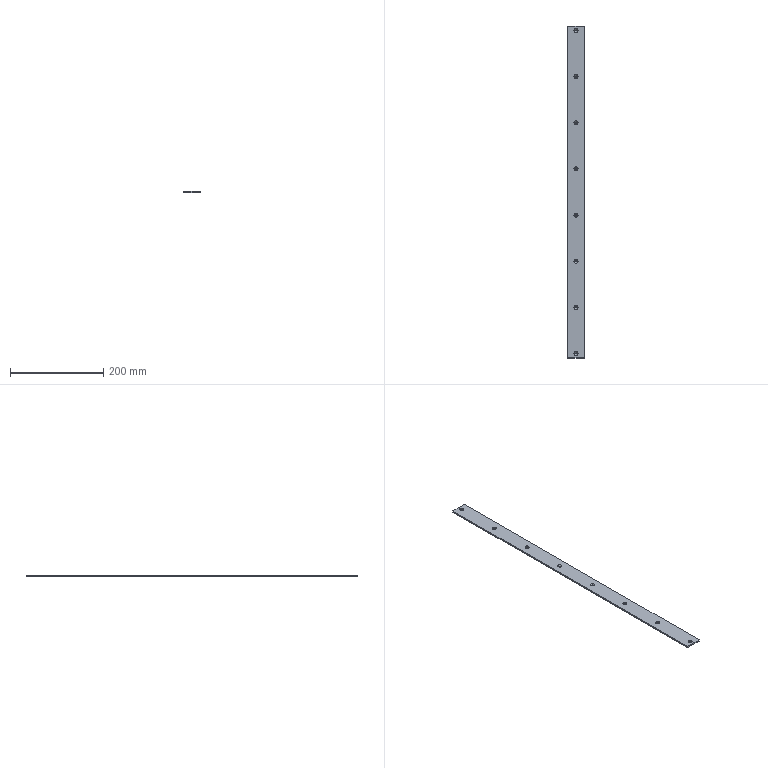Part | SolidWorks | features BaseBody 1 | 1 solid | 38 faces | box 35 x 712 x 3.2 mm | volume 79027 mm3 | cylinder 16 | cone 16 | plane 6 | commonest cylinder face diameters 4.5 x16
STEP:
#1=CARTESIAN_POINT('',(15.25,702.5,-3.2));
#2=VERTEX_POINT('',#1);
#3=CARTESIAN_POINT('',(19.75,702.5,-3.2));
#4=VERTEX_POINT('',#3);
#5=CARTESIAN_POINT('',(17.5,702.5,-3.2));
#6=DIRECTION('',(0.,0.,1.));
#7=DIRECTION('',(1.,0.,0.));
#8=AXIS2_PLACEMENT_3D('',#5,#6,#7);
#9=CIRCLE('',#8,2.25);
#10=EDGE_CURVE('',#2,#4,#9,.T.);
#11=ORIENTED_EDGE('',*,*,#10,.F.);
#12=CARTESIAN_POINT('',(15.25,702.5,-2.05));
#13=VERTEX_POINT('',#12);
#14=CARTESIAN_POINT('',(15.25,702.5,0.));
#15=DIRECTION('',(0.,0.,1.));
#16=VECTOR('',#15,1000.);
#17=LINE('',#14,#16);
#18=EDGE_CURVE('',#2,#13,#17,.T.);
#19=ORIENTED_EDGE('',*,*,#18,.T.);
#20=CARTESIAN_POINT('',(19.75,702.5,-2.05));
#21=VERTEX_POINT('',#20);
#22=CARTESIAN_POINT('',(17.5,702.5,-2.05));
#23=DIRECTION('',(0.,0.,-1.));
#24=DIRECTION('',(1.,0.,0.));
#25=AXIS2_PLACEMENT_3D('',#22,#23,#24);
#26=CIRCLE('',#25,2.25);
#27=EDGE_CURVE('',#21,#13,#26,.T.);
#28=ORIENTED_EDGE('',*,*,#27,.F.);
#29=CARTESIAN_POINT('',(19.75,702.5,0.));
#30=DIRECTION('',(0.,0.,1.));
#31=VECTOR('',#30,1000.);
#32=LINE('',#29,#31);
#33=EDGE_CURVE('',#4,#21,#32,.T.);
#34=ORIENTED_EDGE('',*,*,#33,.F.);
#35=EDGE_LOOP('',(#11,#19,#28,#34));
#36=FACE_OUTER_BOUND('',#35,.T.);
#37=CARTESIAN_POINT('',(17.5,702.5,0.));
#38=DIRECTION('',(0.,0.,1.));
#39=DIRECTION('',(1.,0.,0.));
#40=AXIS2_PLACEMENT_3D('',#37,#38,#39);
#41=CYLINDRICAL_SURFACE('',#40,2.25);
#42=ADVANCED_FACE('',(#36),#41,.F.);
#43=CARTESIAN_POINT('',(15.25,603.5,-3.2));
#44=VERTEX_POINT('',#43);
#45=CARTESIAN_POINT('',(19.75,603.5,-3.2));
#46=VERTEX_POINT('',#45);
#47=CARTESIAN_POINT('',(17.5,603.5,-3.2));
#48=DIRECTION('',(0.,0.,1.));
#49=DIRECTION('',(1.,0.,0.));
#50=AXIS2_PLACEMENT_3D('',#47,#48,#49);
#51=CIRCLE('',#50,2.25);
#52=EDGE_CURVE('',#44,#46,#51,.T.);
#53=ORIENTED_EDGE('',*,*,#52,.F.);
#54=CARTESIAN_POINT('',(15.25,603.5,-2.05));
#55=VERTEX_POINT('',#54);
#56=CARTESIAN_POINT('',(15.25,603.5,0.));
#57=DIRECTION('',(0.,0.,1.));
#58=VECTOR('',#57,1000.);
#59=LINE('',#56,#58);
#60=EDGE_CURVE('',#44,#55,#59,.T.);
#61=ORIENTED_EDGE('',*,*,#60,.T.);
#62=CARTESIAN_POINT('',(19.75,603.5,-2.05));
#63=VERTEX_POINT('',#62);
#64=CARTESIAN_POINT('',(17.5,603.5,-2.05));
#65=DIRECTION('',(0.,0.,-1.));
#66=DIRECTION('',(1.,0.,0.));
#67=AXIS2_PLACEMENT_3D('',#64,#65,#66);
#68=CIRCLE('',#67,2.25);
#69=EDGE_CURVE('',#63,#55,#68,.T.);
#70=ORIENTED_EDGE('',*,*,#69,.F.);
#71=CARTESIAN_POINT('',(19.75,603.5,0.));
#72=DIRECTION('',(0.,0.,1.));
#73=VECTOR('',#72,1000.);
#74=LINE('',#71,#73);
#75=EDGE_CURVE('',#46,#63,#74,.T.);
#76=ORIENTED_EDGE('',*,*,#75,.F.);
#77=EDGE_LOOP('',(#53,#61,#70,#76));
#78=FACE_OUTER_BOUND('',#77,.T.);
#79=CARTESIAN_POINT('',(17.5,603.5,0.));
#80=DIRECTION('',(0.,0.,1.));
#81=DIRECTION('',(1.,0.,0.));
#82=AXIS2_PLACEMENT_3D('',#79,#80,#81);
#83=CYLINDRICAL_SURFACE('',#82,2.25);
#84=ADVANCED_FACE('',(#78),#83,.F.);
#85=CARTESIAN_POINT('',(15.25,504.5,-3.2));
#86=VERTEX_POINT('',#85);
#87=CARTESIAN_POINT('',(19.75,504.5,-3.2));
#88=VERTEX_POINT('',#87);
#89=CARTESIAN_POINT('',(17.5,504.5,-3.2));
#90=DIRECTION('',(0.,0.,1.));
#91=DIRECTION('',(1.,0.,0.));
#92=AXIS2_PLACEMENT_3D('',#89,#90,#91);
#93=CIRCLE('',#92,2.25);
#94=EDGE_CURVE('',#86,#88,#93,.T.);
#95=ORIENTED_EDGE('',*,*,#94,.F.);
#96=CARTESIAN_POINT('',(15.25,504.5,-2.05));
#97=VERTEX_POINT('',#96);
#98=CARTESIAN_POINT('',(15.25,504.5,0.));
#99=DIRECTION('',(0.,0.,1.));
#100=VECTOR('',#99,1000.);
#101=LINE('',#98,#100);
#102=EDGE_CURVE('',#86,#97,#101,.T.);
#103=ORIENTED_EDGE('',*,*,#102,.T.);
#104=CARTESIAN_POINT('',(19.75,504.5,-2.05));
#105=VERTEX_POINT('',#104);
#106=CARTESIAN_POINT('',(17.5,504.5,-2.05));
#107=DIRECTION('',(0.,0.,-1.));
#108=DIRECTION('',(1.,0.,0.));
#109=AXIS2_PLACEMENT_3D('',#106,#107,#108);
#110=CIRCLE('',#109,2.25);
#111=EDGE_CURVE('',#105,#97,#110,.T.);
#112=ORIENTED_EDGE('',*,*,#111,.F.);
#113=CARTESIAN_POINT('',(19.75,504.5,0.));
#114=DIRECTION('',(0.,0.,1.));
#115=VECTOR('',#114,1000.);
#116=LINE('',#113,#115);
#117=EDGE_CURVE('',#88,#105,#116,.T.);
#118=ORIENTED_EDGE('',*,*,#117,.F.);
#119=EDGE_LOOP('',(#95,#103,#112,#118));
#120=FACE_OUTER_BOUND('',#119,.T.);
#121=CARTESIAN_POINT('',(17.5,504.5,0.));
#122=DIRECTION('',(0.,0.,1.));
#123=DIRECTION('',(1.,0.,0.));
#124=AXIS2_PLACEMENT_3D('',#121,#122,#123);
#125=CYLINDRICAL_SURFACE('',#124,2.25);
#126=ADVANCED_FACE('',(#120),#125,.F.);
#127=CARTESIAN_POINT('',(15.25,405.5,-3.2));
#128=VERTEX_POINT('',#127);
#129=CARTESIAN_POINT('',(19.75,405.5,-3.2));
#130=VERTEX_POINT('',#129);
#131=CARTESIAN_POINT('',(17.5,405.5,-3.2));
#132=DIRECTION('',(0.,0.,1.));
#133=DIRECTION('',(1.,0.,0.));
#134=AXIS2_PLACEMENT_3D('',#131,#132,#133);
#135=CIRCLE('',#134,2.25);
#136=EDGE_CURVE('',#128,#130,#135,.T.);
#137=ORIENTED_EDGE('',*,*,#136,.F.);
#138=CARTESIAN_POINT('',(15.25,405.5,-2.05));
#139=VERTEX_POINT('',#138);
#140=CARTESIAN_POINT('',(15.25,405.5,0.));
#141=DIRECTION('',(0.,0.,1.));
#142=VECTOR('',#141,1000.);
#143=LINE('',#140,#142);
#144=EDGE_CURVE('',#128,#139,#143,.T.);
#145=ORIENTED_EDGE('',*,*,#144,.T.);
#146=CARTESIAN_POINT('',(19.75,405.5,-2.05));
#147=VERTEX_POINT('',#146);
#148=CARTESIAN_POINT('',(17.5,405.5,-2.05));
#149=DIRECTION('',(0.,0.,-1.));
#150=DIRECTION('',(1.,0.,0.));
#151=AXIS2_PLACEMENT_3D('',#148,#149,#150);
#152=CIRCLE('',#151,2.25);
#153=EDGE_CURVE('',#147,#139,#152,.T.);
#154=ORIENTED_EDGE('',*,*,#153,.F.);
#155=CARTESIAN_POINT('',(19.75,405.5,0.));
#156=DIRECTION('',(0.,0.,1.));
#157=VECTOR('',#156,1000.);
#158=LINE('',#155,#157);
#159=EDGE_CURVE('',#130,#147,#158,.T.);
#160=ORIENTED_EDGE('',*,*,#159,.F.);
#161=EDGE_LOOP('',(#137,#145,#154,#160));
#162=FACE_OUTER_BOUND('',#161,.T.);
#163=CARTESIAN_POINT('',(17.5,405.5,0.));
#164=DIRECTION('',(0.,0.,1.));
#165=DIRECTION('',(1.,0.,0.));
#166=AXIS2_PLACEMENT_3D('',#163,#164,#165);
#167=CYLINDRICAL_SURFACE('',#166,2.25);
#168=ADVANCED_FACE('',(#162),#167,.F.);
#169=CARTESIAN_POINT('',(15.25,306.5,-3.2));
#170=VERTEX_POINT('',#169);
#171=CARTESIAN_POINT('',(19.75,306.5,-3.2));
#172=VERTEX_POINT('',#171);
#173=CARTESIAN_POINT('',(17.5,306.5,-3.2));
#174=DIRECTION('',(0.,0.,1.));
#175=DIRECTION('',(1.,0.,0.));
#176=AXIS2_PLACEMENT_3D('',#173,#174,#175);
#177=CIRCLE('',#176,2.25);
#178=EDGE_CURVE('',#170,#172,#177,.T.);
#179=ORIENTED_EDGE('',*,*,#178,.F.);
#180=CARTESIAN_POINT('',(15.25,306.5,-2.05));
#181=VERTEX_POINT('',#180);
#182=CARTESIAN_POINT('',(15.25,306.5,0.));
#183=DIRECTION('',(0.,0.,1.));
#184=VECTOR('',#183,1000.);
#185=LINE('',#182,#184);
#186=EDGE_CURVE('',#170,#181,#185,.T.);
#187=ORIENTED_EDGE('',*,*,#186,.T.);
#188=CARTESIAN_POINT('',(19.75,306.5,-2.05));
#189=VERTEX_POINT('',#188);
#190=CARTESIAN_POINT('',(17.5,306.5,-2.05));
#191=DIRECTION('',(0.,0.,-1.));
#192=DIRECTION('',(1.,0.,0.));
#193=AXIS2_PLACEMENT_3D('',#190,#191,#192);
#194=CIRCLE('',#193,2.25);
#195=EDGE_CURVE('',#189,#181,#194,.T.);
#196=ORIENTED_EDGE('',*,*,#195,.F.);
#197=CARTESIAN_POINT('',(19.75,306.5,0.));
#198=DIRECTION('',(0.,0.,1.));
#199=VECTOR('',#198,1000.);
#200=LINE('',#197,#199);
#201=EDGE_CURVE('',#172,#189,#200,.T.);
#202=ORIENTED_EDGE('',*,*,#201,.F.);
#203=EDGE_LOOP('',(#179,#187,#196,#202));
#204=FACE_OUTER_BOUND('',#203,.T.);
#205=CARTESIAN_POINT('',(17.5,306.5,0.));
#206=DIRECTION('',(0.,0.,1.));
#207=DIRECTION('',(1.,0.,0.));
#208=AXIS2_PLACEMENT_3D('',#205,#206,#207);
#209=CYLINDRICAL_SURFACE('',#208,2.25);
#210=ADVANCED_FACE('',(#204),#209,.F.);
#211=CARTESIAN_POINT('',(15.25,207.5,-3.2));
#212=VERTEX_POINT('',#211);
#213=CARTESIAN_POINT('',(19.75,207.5,-3.2));
#214=VERTEX_POINT('',#213);
#215=CARTESIAN_POINT('',(17.5,207.5,-3.2));
#216=DIRECTION('',(0.,0.,1.));
#217=DIRECTION('',(1.,0.,0.));
#218=AXIS2_PLACEMENT_3D('',#215,#216,#217);
#219=CIRCLE('',#218,2.25);
#220=EDGE_CURVE('',#212,#214,#219,.T.);
#221=ORIENTED_EDGE('',*,*,#220,.F.);
#222=CARTESIAN_POINT('',(15.25,207.5,-2.05));
#223=VERTEX_POINT('',#222);
#224=CARTESIAN_POINT('',(15.25,207.5,0.));
#225=DIRECTION('',(0.,0.,1.));
#226=VECTOR('',#225,1000.);
#227=LINE('',#224,#226);
#228=EDGE_CURVE('',#212,#223,#227,.T.);
#229=ORIENTED_EDGE('',*,*,#228,.T.);
#230=CARTESIAN_POINT('',(19.75,207.5,-2.05));
#231=VERTEX_POINT('',#230);
#232=CARTESIAN_POINT('',(17.5,207.5,-2.05));
#233=DIRECTION('',(0.,0.,-1.));
#234=DIRECTION('',(1.,0.,0.));
#235=AXIS2_PLACEMENT_3D('',#232,#233,#234);
#236=CIRCLE('',#235,2.25);
#237=EDGE_CURVE('',#231,#223,#236,.T.);
#238=ORIENTED_EDGE('',*,*,#237,.F.);
#239=CARTESIAN_POINT('',(19.75,207.5,0.));
#240=DIRECTION('',(0.,0.,1.));
#241=VECTOR('',#240,1000.);
#242=LINE('',#239,#241);
#243=EDGE_CURVE('',#214,#231,#242,.T.);
#244=ORIENTED_EDGE('',*,*,#243,.F.);
#245=EDGE_LOOP('',(#221,#229,#238,#244));
#246=FACE_OUTER_BOUND('',#245,.T.);
#247=CARTESIAN_POINT('',(17.5,207.5,0.));
#248=DIRECTION('',(0.,0.,1.));
#249=DIRECTION('',(1.,0.,0.));
#250=AXIS2_PLACEMENT_3D('',#247,#248,#249);
#251=CYLINDRICAL_SURFACE('',#250,2.25);
#252=ADVANCED_FACE('',(#246),#251,.F.);
#253=CARTESIAN_POINT('',(15.25,9.5,-3.2));
#254=VERTEX_POINT('',#253);
#255=CARTESIAN_POINT('',(19.75,9.5,-3.2));
#256=VERTEX_POINT('',#255);
#257=CARTESIAN_POINT('',(17.5,9.5,-3.2));
#258=DIRECTION('',(0.,0.,1.));
#259=DIRECTION('',(1.,0.,0.));
#260=AXIS2_PLACEMENT_3D('',#257,#258,#259);
#261=CIRCLE('',#260,2.25);
#262=EDGE_CURVE('',#254,#256,#261,.T.);
#263=ORIENTED_EDGE('',*,*,#262,.F.);
#264=CARTESIAN_POINT('',(15.25,9.5,-2.05));
#265=VERTEX_POINT('',#264);
#266=CARTESIAN_POINT('',(15.25,9.5,0.));
#267=DIRECTION('',(0.,0.,1.));
#268=VECTOR('',#267,1000.);
#269=LINE('',#266,#268);
#270=EDGE_CURVE('',#254,#265,#269,.T.);
#271=ORIENTED_EDGE('',*,*,#270,.T.);
#272=CARTESIAN_POINT('',(19.75,9.5,-2.05));
#273=VERTEX_POINT('',#272);
#274=CARTESIAN_POINT('',(17.5,9.5,-2.05));
#275=DIRECTION('',(0.,0.,-1.));
#276=DIRECTION('',(1.,0.,0.));
#277=AXIS2_PLACEMENT_3D('',#274,#275,#276);
#278=CIRCLE('',#277,2.25);
#279=EDGE_CURVE('',#273,#265,#278,.T.);
#280=ORIENTED_EDGE('',*,*,#279,.F.);
#281=CARTESIAN_POINT('',(19.75,9.5,0.));
#282=DIRECTION('',(0.,0.,1.));
#283=VECTOR('',#282,1000.);
#284=LINE('',#281,#283);
#285=EDGE_CURVE('',#256,#273,#284,.T.);
#286=ORIENTED_EDGE('',*,*,#285,.F.);
#287=EDGE_LOOP('',(#263,#271,#280,#286));
#288=FACE_OUTER_BOUND('',#287,.T.);
#289=CARTESIAN_POINT('',(17.5,9.5,0.));
#290=DIRECTION('',(0.,0.,1.));
#291=DIRECTION('',(1.,0.,0.));
#292=AXIS2_PLACEMENT_3D('',#289,#290,#291);
#293=CYLINDRICAL_SURFACE('',#292,2.25);
#294=ADVANCED_FACE('',(#288),#293,.F.);
#295=CARTESIAN_POINT('',(15.25,108.5,-3.2));
#296=VERTEX_POINT('',#295);
#297=CARTESIAN_POINT('',(19.75,108.5,-3.2));
#298=VERTEX_POINT('',#297);
#299=CARTESIAN_POINT('',(17.5,108.5,-3.2));
#300=DIRECTION('',(0.,0.,1.));
#301=DIRECTION('',(1.,0.,0.));
#302=AXIS2_PLACEMENT_3D('',#299,#300,#301);
#303=CIRCLE('',#302,2.25);
#304=EDGE_CURVE('',#296,#298,#303,.T.);
#305=ORIENTED_EDGE('',*,*,#304,.F.);
#306=CARTESIAN_POINT('',(15.25,108.5,-2.05));
#307=VERTEX_POINT('',#306);
#308=CARTESIAN_POINT('',(15.25,108.5,0.));
#309=DIRECTION('',(0.,0.,1.));
#310=VECTOR('',#309,1000.);
#311=LINE('',#308,#310);
#312=EDGE_CURVE('',#296,#307,#311,.T.);
#313=ORIENTED_EDGE('',*,*,#312,.T.);
#314=CARTESIAN_POINT('',(19.75,108.5,-2.05));
#315=VERTEX_POINT('',#314);
#316=CARTESIAN_POINT('',(17.5,108.5,-2.05));
#317=DIRECTION('',(0.,0.,-1.));
#318=DIRECTION('',(1.,0.,0.));
#319=AXIS2_PLACEMENT_3D('',#316,#317,#318);
#320=CIRCLE('',#319,2.25);
#321=EDGE_CURVE('',#315,#307,#320,.T.);
#322=ORIENTED_EDGE('',*,*,#321,.F.);
#323=CARTESIAN_POINT('',(19.75,108.5,0.));
#324=DIRECTION('',(0.,0.,1.));
#325=VECTOR('',#324,1000.);
#326=LINE('',#323,#325);
#327=EDGE_CURVE('',#298,#315,#326,.T.);
#328=ORIENTED_EDGE('',*,*,#327,.F.);
#329=EDGE_LOOP('',(#305,#313,#322,#328));
#330=FACE_OUTER_BOUND('',#329,.T.);
#331=CARTESIAN_POINT('',(17.5,108.5,0.));
#332=DIRECTION('',(0.,0.,1.));
#333=DIRECTION('',(1.,0.,0.));
#334=AXIS2_PLACEMENT_3D('',#331,#332,#333);
#335=CYLINDRICAL_SURFACE('',#334,2.25);
#336=ADVANCED_FACE('',(#330),#335,.F.);
#337=ORIENTED_EDGE('',*,*,#27,.T.);
#338=CARTESIAN_POINT('',(13.2,702.5,0.));
#339=VERTEX_POINT('',#338);
#340=CARTESIAN_POINT('',(13.2,702.5,0.));
#341=DIRECTION('',(-0.7071,0.,0.7071));
#342=VECTOR('',#341,1000.);
#343=LINE('',#340,#342);
#344=EDGE_CURVE('',#13,#339,#343,.T.);
#345=ORIENTED_EDGE('',*,*,#344,.T.);
#346=CARTESIAN_POINT('',(21.8,702.5,0.));
#347=VERTEX_POINT('',#346);
#348=CARTESIAN_POINT('',(17.5,702.5,0.));
#349=DIRECTION('',(0.,0.,-1.));
#350=DIRECTION('',(1.,0.,0.));
#351=AXIS2_PLACEMENT_3D('',#348,#349,#350);
#352=CIRCLE('',#351,4.3);
#353=EDGE_CURVE('',#347,#339,#352,.T.);
#354=ORIENTED_EDGE('',*,*,#353,.F.);
#355=CARTESIAN_POINT('',(21.8,702.5,0.));
#356=DIRECTION('',(0.7071,0.,0.7071));
#357=VECTOR('',#356,1000.);
#358=LINE('',#355,#357);
#359=EDGE_CURVE('',#21,#347,#358,.T.);
#360=ORIENTED_EDGE('',*,*,#359,.F.);
#361=EDGE_LOOP('',(#337,#345,#354,#360));
#362=FACE_OUTER_BOUND('',#361,.T.);
#363=CARTESIAN_POINT('',(17.5,702.5,0.));
#364=DIRECTION('',(0.,0.,1.));
#365=DIRECTION('',(1.,0.,0.));
#366=AXIS2_PLACEMENT_3D('',#363,#364,#365);
#367=CONICAL_SURFACE('',#366,4.3,0.7854);
#368=ADVANCED_FACE('',(#362),#367,.F.);
#369=ORIENTED_EDGE('',*,*,#69,.T.);
#370=CARTESIAN_POINT('',(13.2,603.5,0.));
#371=VERTEX_POINT('',#370);
#372=CARTESIAN_POINT('',(13.2,603.5,0.));
#373=DIRECTION('',(-0.7071,0.,0.7071));
#374=VECTOR('',#373,1000.);
#375=LINE('',#372,#374);
#376=EDGE_CURVE('',#55,#371,#375,.T.);
#377=ORIENTED_EDGE('',*,*,#376,.T.);
#378=CARTESIAN_POINT('',(21.8,603.5,0.));
#379=VERTEX_POINT('',#378);
#380=CARTESIAN_POINT('',(17.5,603.5,0.));
#381=DIRECTION('',(0.,0.,-1.));
#382=DIRECTION('',(1.,0.,0.));
#383=AXIS2_PLACEMENT_3D('',#380,#381,#382);
#384=CIRCLE('',#383,4.3);
#385=EDGE_CURVE('',#379,#371,#384,.T.);
#386=ORIENTED_EDGE('',*,*,#385,.F.);
#387=CARTESIAN_POINT('',(21.8,603.5,0.));
#388=DIRECTION('',(0.7071,0.,0.7071));
#389=VECTOR('',#388,1000.);
#390=LINE('',#387,#389);
#391=EDGE_CURVE('',#63,#379,#390,.T.);
#392=ORIENTED_EDGE('',*,*,#391,.F.);
#393=EDGE_LOOP('',(#369,#377,#386,#392));
#394=FACE_OUTER_BOUND('',#393,.T.);
#395=CARTESIAN_POINT('',(17.5,603.5,0.));
#396=DIRECTION('',(0.,0.,1.));
#397=DIRECTION('',(1.,0.,0.));
#398=AXIS2_PLACEMENT_3D('',#395,#396,#397);
#399=CONICAL_SURFACE('',#398,4.3,0.7854);
#400=ADVANCED_FACE('',(#394),#399,.F.);
#401=ORIENTED_EDGE('',*,*,#111,.T.);
#402=CARTESIAN_POINT('',(13.2,504.5,0.));
#403=VERTEX_POINT('',#402);
#404=CARTESIAN_POINT('',(13.2,504.5,0.));
#405=DIRECTION('',(-0.7071,0.,0.7071));
#406=VECTOR('',#405,1000.);
#407=LINE('',#404,#406);
#408=EDGE_CURVE('',#97,#403,#407,.T.);
#409=ORIENTED_EDGE('',*,*,#408,.T.);
#410=CARTESIAN_POINT('',(21.8,504.5,0.));
#411=VERTEX_POINT('',#410);
#412=CARTESIAN_POINT('',(17.5,504.5,0.));
#413=DIRECTION('',(0.,0.,-1.));
#414=DIRECTION('',(1.,0.,0.));
#415=AXIS2_PLACEMENT_3D('',#412,#413,#414);
#416=CIRCLE('',#415,4.3);
#417=EDGE_CURVE('',#411,#403,#416,.T.);
#418=ORIENTED_EDGE('',*,*,#417,.F.);
#419=CARTESIAN_POINT('',(21.8,504.5,0.));
#420=DIRECTION('',(0.7071,0.,0.7071));
#421=VECTOR('',#420,1000.);
#422=LINE('',#419,#421);
#423=EDGE_CURVE('',#105,#411,#422,.T.);
#424=ORIENTED_EDGE('',*,*,#423,.F.);
#425=EDGE_LOOP('',(#401,#409,#418,#424));
#426=FACE_OUTER_BOUND('',#425,.T.);
#427=CARTESIAN_POINT('',(17.5,504.5,0.));
#428=DIRECTION('',(0.,0.,1.));
#429=DIRECTION('',(1.,0.,0.));
#430=AXIS2_PLACEMENT_3D('',#427,#428,#429);
#431=CONICAL_SURFACE('',#430,4.3,0.7854);
#432=ADVANCED_FACE('',(#426),#431,.F.);
#433=ORIENTED_EDGE('',*,*,#153,.T.);
#434=CARTESIAN_POINT('',(13.2,405.5,0.));
#435=VERTEX_POINT('',#434);
#436=CARTESIAN_POINT('',(13.2,405.5,0.));
#437=DIRECTION('',(-0.7071,0.,0.7071));
#438=VECTOR('',#437,1000.);
#439=LINE('',#436,#438);
#440=EDGE_CURVE('',#139,#435,#439,.T.);
#441=ORIENTED_EDGE('',*,*,#440,.T.);
#442=CARTESIAN_POINT('',(21.8,405.5,0.));
#443=VERTEX_POINT('',#442);
#444=CARTESIAN_POINT('',(17.5,405.5,0.));
#445=DIRECTION('',(0.,0.,-1.));
#446=DIRECTION('',(1.,0.,0.));
#447=AXIS2_PLACEMENT_3D('',#444,#445,#446);
#448=CIRCLE('',#447,4.3);
#449=EDGE_CURVE('',#443,#435,#448,.T.);
#450=ORIENTED_EDGE('',*,*,#449,.F.);
#451=CARTESIAN_POINT('',(21.8,405.5,0.));
#452=DIRECTION('',(0.7071,0.,0.7071));
#453=VECTOR('',#452,1000.);
#454=LINE('',#451,#453);
#455=EDGE_CURVE('',#147,#443,#454,.T.);
#456=ORIENTED_EDGE('',*,*,#455,.F.);
#457=EDGE_LOOP('',(#433,#441,#450,#456));
#458=FACE_OUTER_BOUND('',#457,.T.);
#459=CARTESIAN_POINT('',(17.5,405.5,0.));
#460=DIRECTION('',(0.,0.,1.));
#461=DIRECTION('',(1.,0.,0.));
#462=AXIS2_PLACEMENT_3D('',#459,#460,#461);
#463=CONICAL_SURFACE('',#462,4.3,0.7854);
#464=ADVANCED_FACE('',(#458),#463,.F.);
#465=ORIENTED_EDGE('',*,*,#195,.T.);
#466=CARTESIAN_POINT('',(13.2,306.5,0.));
#467=VERTEX_POINT('',#466);
#468=CARTESIAN_POINT('',(13.2,306.5,0.));
#469=DIRECTION('',(-0.7071,0.,0.7071));
#470=VECTOR('',#469,1000.);
#471=LINE('',#468,#470);
#472=EDGE_CURVE('',#181,#467,#471,.T.);
#473=ORIENTED_EDGE('',*,*,#472,.T.);
#474=CARTESIAN_POINT('',(21.8,306.5,0.));
#475=VERTEX_POINT('',#474);
#476=CARTESIAN_POINT('',(17.5,306.5,0.));
#477=DIRECTION('',(0.,0.,-1.));
#478=DIRECTION('',(1.,0.,0.));
#479=AXIS2_PLACEMENT_3D('',#476,#477,#478);
#480=CIRCLE('',#479,4.3);
#481=EDGE_CURVE('',#475,#467,#480,.T.);
#482=ORIENTED_EDGE('',*,*,#481,.F.);
#483=CARTESIAN_POINT('',(21.8,306.5,0.));
#484=DIRECTION('',(0.7071,0.,0.7071));
#485=VECTOR('',#484,1000.);
#486=LINE('',#483,#485);
#487=EDGE_CURVE('',#189,#475,#486,.T.);
#488=ORIENTED_EDGE('',*,*,#487,.F.);
#489=EDGE_LOOP('',(#465,#473,#482,#488));
#490=FACE_OUTER_BOUND('',#489,.T.);
#491=CARTESIAN_POINT('',(17.5,306.5,0.));
#492=DIRECTION('',(0.,0.,1.));
#493=DIRECTION('',(1.,0.,0.));
#494=AXIS2_PLACEMENT_3D('',#491,#492,#493);
#495=CONICAL_SURFACE('',#494,4.3,0.7854);
#496=ADVANCED_FACE('',(#490),#495,.F.);
#497=ORIENTED_EDGE('',*,*,#237,.T.);
#498=CARTESIAN_POINT('',(13.2,207.5,0.));
#499=VERTEX_POINT('',#498);
#500=CARTESIAN_POINT('',(13.2,207.5,0.));
#501=DIRECTION('',(-0.7071,0.,0.7071));
#502=VECTOR('',#501,1000.);
#503=LINE('',#500,#502);
#504=EDGE_CURVE('',#223,#499,#503,.T.);
#505=ORIENTED_EDGE('',*,*,#504,.T.);
#506=CARTESIAN_POINT('',(21.8,207.5,0.));
#507=VERTEX_POINT('',#506);
#508=CARTESIAN_POINT('',(17.5,207.5,0.));
#509=DIRECTION('',(0.,0.,-1.));
#510=DIRECTION('',(1.,0.,0.));
#511=AXIS2_PLACEMENT_3D('',#508,#509,#510);
#512=CIRCLE('',#511,4.3);
#513=EDGE_CURVE('',#507,#499,#512,.T.);
#514=ORIENTED_EDGE('',*,*,#513,.F.);
#515=CARTESIAN_POINT('',(21.8,207.5,0.));
#516=DIRECTION('',(0.7071,0.,0.7071));
#517=VECTOR('',#516,1000.);
#518=LINE('',#515,#517);
#519=EDGE_CURVE('',#231,#507,#518,.T.);
#520=ORIENTED_EDGE('',*,*,#519,.F.);
#521=EDGE_LOOP('',(#497,#505,#514,#520));
#522=FACE_OUTER_BOUND('',#521,.T.);
#523=CARTESIAN_POINT('',(17.5,207.5,0.));
#524=DIRECTION('',(0.,0.,1.));
#525=DIRECTION('',(1.,0.,0.));
#526=AXIS2_PLACEMENT_3D('',#523,#524,#525);
#527=CONICAL_SURFACE('',#526,4.3,0.7854);
#528=ADVANCED_FACE('',(#522),#527,.F.);
#529=ORIENTED_EDGE('',*,*,#279,.T.);
#530=CARTESIAN_POINT('',(13.2,9.5,0.));
#531=VERTEX_POINT('',#530);
#532=CARTESIAN_POINT('',(13.2,9.5,0.));
#533=DIRECTION('',(-0.7071,0.,0.7071));
#534=VECTOR('',#533,1000.);
#535=LINE('',#532,#534);
#536=EDGE_CURVE('',#265,#531,#535,.T.);
#537=ORIENTED_EDGE('',*,*,#536,.T.);
#538=CARTESIAN_POINT('',(21.8,9.5,0.));
#539=VERTEX_POINT('',#538);
#540=CARTESIAN_POINT('',(17.5,9.5,0.));
#541=DIRECTION('',(0.,0.,1.));
#542=DIRECTION('',(1.,0.,0.));
#543=AXIS2_PLACEMENT_3D('',#540,#541,#542);
#544=CIRCLE('',#543,4.3);
#545=EDGE_CURVE('',#531,#539,#544,.T.);
#546=ORIENTED_EDGE('',*,*,#545,.T.);
#547=CARTESIAN_POINT('',(21.8,9.5,0.));
#548=DIRECTION('',(0.7071,0.,0.7071));
#549=VECTOR('',#548,1000.);
#550=LINE('',#547,#549);
#551=EDGE_CURVE('',#273,#539,#550,.T.);
#552=ORIENTED_EDGE('',*,*,#551,.F.);
#553=EDGE_LOOP('',(#529,#537,#546,#552));
#554=FACE_OUTER_BOUND('',#553,.T.);
#555=CARTESIAN_POINT('',(17.5,9.5,0.));
#556=DIRECTION('',(0.,0.,1.));
#557=DIRECTION('',(1.,0.,0.));
#558=AXIS2_PLACEMENT_3D('',#555,#556,#557);
#559=CONICAL_SURFACE('',#558,4.3,0.7854);
#560=ADVANCED_FACE('',(#554),#559,.F.);
#561=ORIENTED_EDGE('',*,*,#321,.T.);
#562=CARTESIAN_POINT('',(13.2,108.5,0.));
#563=VERTEX_POINT('',#562);
#564=CARTESIAN_POINT('',(13.2,108.5,0.));
#565=DIRECTION('',(-0.7071,0.,0.7071));
#566=VECTOR('',#565,1000.);
#567=LINE('',#564,#566);
#568=EDGE_CURVE('',#307,#563,#567,.T.);
#569=ORIENTED_EDGE('',*,*,#568,.T.);
#570=CARTESIAN_POINT('',(21.8,108.5,0.));
#571=VERTEX_POINT('',#570);
#572=CARTESIAN_POINT('',(17.5,108.5,0.));
#573=DIRECTION('',(0.,0.,1.));
#574=DIRECTION('',(1.,0.,0.));
#575=AXIS2_PLACEMENT_3D('',#572,#573,#574);
#576=CIRCLE('',#575,4.3);
#577=EDGE_CURVE('',#563,#571,#576,.T.);
#578=ORIENTED_EDGE('',*,*,#577,.T.);
#579=CARTESIAN_POINT('',(21.8,108.5,0.));
#580=DIRECTION('',(0.7071,0.,0.7071));
#581=VECTOR('',#580,1000.);
#582=LINE('',#579,#581);
#583=EDGE_CURVE('',#315,#571,#582,.T.);
#584=ORIENTED_EDGE('',*,*,#583,.F.);
#585=EDGE_LOOP('',(#561,#569,#578,#584));
#586=FACE_OUTER_BOUND('',#585,.T.);
#587=CARTESIAN_POINT('',(17.5,108.5,0.));
#588=DIRECTION('',(0.,0.,1.));
#589=DIRECTION('',(1.,0.,0.));
#590=AXIS2_PLACEMENT_3D('',#587,#588,#589);
#591=CONICAL_SURFACE('',#590,4.3,0.7854);
#592=ADVANCED_FACE('',(#586),#591,.F.);
#593=CARTESIAN_POINT('',(17.5,702.5,-3.2));
#594=DIRECTION('',(0.,0.,1.));
#595=DIRECTION('',(1.,0.,0.));
#596=AXIS2_PLACEMENT_3D('',#593,#594,#595);
#597=CIRCLE('',#596,2.25);
#598=EDGE_CURVE('',#4,#2,#597,.T.);
#599=ORIENTED_EDGE('',*,*,#598,.T.);
#600=ORIENTED_EDGE('',*,*,#10,.T.);
#601=EDGE_LOOP('',(#599,#600));
#602=FACE_BOUND('',#601,.T.);
#603=CARTESIAN_POINT('',(17.5,603.5,-3.2));
#604=DIRECTION('',(0.,0.,1.));
#605=DIRECTION('',(1.,0.,0.));
#606=AXIS2_PLACEMENT_3D('',#603,#604,#605);
#607=CIRCLE('',#606,2.25);
#608=EDGE_CURVE('',#46,#44,#607,.T.);
#609=ORIENTED_EDGE('',*,*,#608,.T.);
#610=ORIENTED_EDGE('',*,*,#52,.T.);
#611=EDGE_LOOP('',(#609,#610));
#612=FACE_BOUND('',#611,.T.);
#613=CARTESIAN_POINT('',(17.5,504.5,-3.2));
#614=DIRECTION('',(0.,0.,1.));
#615=DIRECTION('',(1.,0.,0.));
#616=AXIS2_PLACEMENT_3D('',#613,#614,#615);
#617=CIRCLE('',#616,2.25);
#618=EDGE_CURVE('',#88,#86,#617,.T.);
#619=ORIENTED_EDGE('',*,*,#618,.T.);
#620=ORIENTED_EDGE('',*,*,#94,.T.);
#621=EDGE_LOOP('',(#619,#620));
#622=FACE_BOUND('',#621,.T.);
#623=CARTESIAN_POINT('',(17.5,405.5,-3.2));
#624=DIRECTION('',(0.,0.,1.));
#625=DIRECTION('',(1.,0.,0.));
#626=AXIS2_PLACEMENT_3D('',#623,#624,#625);
#627=CIRCLE('',#626,2.25);
#628=EDGE_CURVE('',#130,#128,#627,.T.);
#629=ORIENTED_EDGE('',*,*,#628,.T.);
#630=ORIENTED_EDGE('',*,*,#136,.T.);
#631=EDGE_LOOP('',(#629,#630));
#632=FACE_BOUND('',#631,.T.);
#633=CARTESIAN_POINT('',(17.5,306.5,-3.2));
#634=DIRECTION('',(0.,0.,1.));
#635=DIRECTION('',(1.,0.,0.));
#636=AXIS2_PLACEMENT_3D('',#633,#634,#635);
#637=CIRCLE('',#636,2.25);
#638=EDGE_CURVE('',#172,#170,#637,.T.);
#639=ORIENTED_EDGE('',*,*,#638,.T.);
#640=ORIENTED_EDGE('',*,*,#178,.T.);
#641=EDGE_LOOP('',(#639,#640));
#642=FACE_BOUND('',#641,.T.);
#643=CARTESIAN_POINT('',(17.5,207.5,-3.2));
#644=DIRECTION('',(0.,0.,1.));
#645=DIRECTION('',(1.,0.,0.));
#646=AXIS2_PLACEMENT_3D('',#643,#644,#645);
#647=CIRCLE('',#646,2.25);
#648=EDGE_CURVE('',#214,#212,#647,.T.);
#649=ORIENTED_EDGE('',*,*,#648,.T.);
#650=ORIENTED_EDGE('',*,*,#220,.T.);
#651=EDGE_LOOP('',(#649,#650));
#652=FACE_BOUND('',#651,.T.);
#653=CARTESIAN_POINT('',(35.,712.,-3.2));
#654=VERTEX_POINT('',#653);
#655=CARTESIAN_POINT('',(35.,0.,-3.2));
#656=VERTEX_POINT('',#655);
#657=CARTESIAN_POINT('',(35.,0.,-3.2));
#658=DIRECTION('',(0.,-1.,0.));
#659=VECTOR('',#658,1000.);
#660=LINE('',#657,#659);
#661=EDGE_CURVE('',#654,#656,#660,.T.);
#662=ORIENTED_EDGE('',*,*,#661,.T.);
#663=CARTESIAN_POINT('',(0.,0.,-3.2));
#664=VERTEX_POINT('',#663);
#665=CARTESIAN_POINT('',(0.,0.,-3.2));
#666=DIRECTION('',(-1.,0.,0.));
#667=VECTOR('',#666,1000.);
#668=LINE('',#665,#667);
#669=EDGE_CURVE('',#656,#664,#668,.T.);
#670=ORIENTED_EDGE('',*,*,#669,.T.);
#671=CARTESIAN_POINT('',(0.,712.,-3.2));
#672=VERTEX_POINT('',#671);
#673=CARTESIAN_POINT('',(0.,0.,-3.2));
#674=DIRECTION('',(0.,1.,0.));
#675=VECTOR('',#674,1000.);
#676=LINE('',#673,#675);
#677=EDGE_CURVE('',#664,#672,#676,.T.);
#678=ORIENTED_EDGE('',*,*,#677,.T.);
#679=CARTESIAN_POINT('',(0.,712.,-3.2));
#680=DIRECTION('',(1.,0.,0.));
#681=VECTOR('',#680,1000.);
#682=LINE('',#679,#681);
#683=EDGE_CURVE('',#672,#654,#682,.T.);
#684=ORIENTED_EDGE('',*,*,#683,.T.);
#685=EDGE_LOOP('',(#662,#670,#678,#684));
#686=FACE_OUTER_BOUND('',#685,.T.);
#687=CARTESIAN_POINT('',(17.5,9.5,-3.2));
#688=DIRECTION('',(0.,0.,1.));
#689=DIRECTION('',(1.,0.,0.));
#690=AXIS2_PLACEMENT_3D('',#687,#688,#689);
#691=CIRCLE('',#690,2.25);
#692=EDGE_CURVE('',#256,#254,#691,.T.);
#693=ORIENTED_EDGE('',*,*,#692,.T.);
#694=ORIENTED_EDGE('',*,*,#262,.T.);
#695=EDGE_LOOP('',(#693,#694));
#696=FACE_BOUND('',#695,.T.);
#697=CARTESIAN_POINT('',(17.5,108.5,-3.2));
#698=DIRECTION('',(0.,0.,1.));
#699=DIRECTION('',(1.,0.,0.));
#700=AXIS2_PLACEMENT_3D('',#697,#698,#699);
#701=CIRCLE('',#700,2.25);
#702=EDGE_CURVE('',#298,#296,#701,.T.);
#703=ORIENTED_EDGE('',*,*,#702,.T.);
#704=ORIENTED_EDGE('',*,*,#304,.T.);
#705=EDGE_LOOP('',(#703,#704));
#706=FACE_BOUND('',#705,.T.);
#707=CARTESIAN_POINT('',(0.,0.,-3.2));
#708=DIRECTION('',(0.,0.,-1.));
#709=DIRECTION('',(-1.,0.,0.));
#710=AXIS2_PLACEMENT_3D('',#707,#708,#709);
#711=PLANE('',#710);
#712=ADVANCED_FACE('',(#602,#612,#622,#632,#642,#652,#686,#696,#706),#711,.T.);
#713=ORIENTED_EDGE('',*,*,#18,.F.);
#714=ORIENTED_EDGE('',*,*,#598,.F.);
#715=ORIENTED_EDGE('',*,*,#33,.T.);
#716=CARTESIAN_POINT('',(17.5,702.5,-2.05));
#717=DIRECTION('',(0.,0.,-1.));
#718=DIRECTION('',(1.,0.,0.));
#719=AXIS2_PLACEMENT_3D('',#716,#717,#718);
#720=CIRCLE('',#719,2.25);
#721=EDGE_CURVE('',#13,#21,#720,.T.);
#722=ORIENTED_EDGE('',*,*,#721,.F.);
#723=EDGE_LOOP('',(#713,#714,#715,#722));
#724=FACE_OUTER_BOUND('',#723,.T.);
#725=CARTESIAN_POINT('',(17.5,702.5,0.));
#726=DIRECTION('',(0.,0.,1.));
#727=DIRECTION('',(1.,0.,0.));
#728=AXIS2_PLACEMENT_3D('',#725,#726,#727);
#729=CYLINDRICAL_SURFACE('',#728,2.25);
#730=ADVANCED_FACE('',(#724),#729,.F.);
#731=ORIENTED_EDGE('',*,*,#60,.F.);
#732=ORIENTED_EDGE('',*,*,#608,.F.);
#733=ORIENTED_EDGE('',*,*,#75,.T.);
#734=CARTESIAN_POINT('',(17.5,603.5,-2.05));
#735=DIRECTION('',(0.,0.,-1.));
#736=DIRECTION('',(1.,0.,0.));
#737=AXIS2_PLACEMENT_3D('',#734,#735,#736);
#738=CIRCLE('',#737,2.25);
#739=EDGE_CURVE('',#55,#63,#738,.T.);
#740=ORIENTED_EDGE('',*,*,#739,.F.);
#741=EDGE_LOOP('',(#731,#732,#733,#740));
#742=FACE_OUTER_BOUND('',#741,.T.);
#743=CARTESIAN_POINT('',(17.5,603.5,0.));
#744=DIRECTION('',(0.,0.,1.));
#745=DIRECTION('',(1.,0.,0.));
#746=AXIS2_PLACEMENT_3D('',#743,#744,#745);
#747=CYLINDRICAL_SURFACE('',#746,2.25);
#748=ADVANCED_FACE('',(#742),#747,.F.);
#749=ORIENTED_EDGE('',*,*,#102,.F.);
#750=ORIENTED_EDGE('',*,*,#618,.F.);
#751=ORIENTED_EDGE('',*,*,#117,.T.);
#752=CARTESIAN_POINT('',(17.5,504.5,-2.05));
#753=DIRECTION('',(0.,0.,-1.));
#754=DIRECTION('',(1.,0.,0.));
#755=AXIS2_PLACEMENT_3D('',#752,#753,#754);
#756=CIRCLE('',#755,2.25);
#757=EDGE_CURVE('',#97,#105,#756,.T.);
#758=ORIENTED_EDGE('',*,*,#757,.F.);
#759=EDGE_LOOP('',(#749,#750,#751,#758));
#760=FACE_OUTER_BOUND('',#759,.T.);
#761=CARTESIAN_POINT('',(17.5,504.5,0.));
#762=DIRECTION('',(0.,0.,1.));
#763=DIRECTION('',(1.,0.,0.));
#764=AXIS2_PLACEMENT_3D('',#761,#762,#763);
#765=CYLINDRICAL_SURFACE('',#764,2.25);
#766=ADVANCED_FACE('',(#760),#765,.F.);
#767=ORIENTED_EDGE('',*,*,#144,.F.);
#768=ORIENTED_EDGE('',*,*,#628,.F.);
#769=ORIENTED_EDGE('',*,*,#159,.T.);
#770=CARTESIAN_POINT('',(17.5,405.5,-2.05));
#771=DIRECTION('',(0.,0.,-1.));
#772=DIRECTION('',(1.,0.,0.));
#773=AXIS2_PLACEMENT_3D('',#770,#771,#772);
#774=CIRCLE('',#773,2.25);
#775=EDGE_CURVE('',#139,#147,#774,.T.);
#776=ORIENTED_EDGE('',*,*,#775,.F.);
#777=EDGE_LOOP('',(#767,#768,#769,#776));
#778=FACE_OUTER_BOUND('',#777,.T.);
#779=CARTESIAN_POINT('',(17.5,405.5,0.));
#780=DIRECTION('',(0.,0.,1.));
#781=DIRECTION('',(1.,0.,0.));
#782=AXIS2_PLACEMENT_3D('',#779,#780,#781);
#783=CYLINDRICAL_SURFACE('',#782,2.25);
#784=ADVANCED_FACE('',(#778),#783,.F.);
#785=ORIENTED_EDGE('',*,*,#186,.F.);
#786=ORIENTED_EDGE('',*,*,#638,.F.);
#787=ORIENTED_EDGE('',*,*,#201,.T.);
#788=CARTESIAN_POINT('',(17.5,306.5,-2.05));
#789=DIRECTION('',(0.,0.,-1.));
#790=DIRECTION('',(1.,0.,0.));
#791=AXIS2_PLACEMENT_3D('',#788,#789,#790);
#792=CIRCLE('',#791,2.25);
#793=EDGE_CURVE('',#181,#189,#792,.T.);
#794=ORIENTED_EDGE('',*,*,#793,.F.);
#795=EDGE_LOOP('',(#785,#786,#787,#794));
#796=FACE_OUTER_BOUND('',#795,.T.);
#797=CARTESIAN_POINT('',(17.5,306.5,0.));
#798=DIRECTION('',(0.,0.,1.));
#799=DIRECTION('',(1.,0.,0.));
#800=AXIS2_PLACEMENT_3D('',#797,#798,#799);
#801=CYLINDRICAL_SURFACE('',#800,2.25);
#802=ADVANCED_FACE('',(#796),#801,.F.);
#803=ORIENTED_EDGE('',*,*,#228,.F.);
#804=ORIENTED_EDGE('',*,*,#648,.F.);
#805=ORIENTED_EDGE('',*,*,#243,.T.);
#806=CARTESIAN_POINT('',(17.5,207.5,-2.05));
#807=DIRECTION('',(0.,0.,-1.));
#808=DIRECTION('',(1.,0.,0.));
#809=AXIS2_PLACEMENT_3D('',#806,#807,#808);
#810=CIRCLE('',#809,2.25);
#811=EDGE_CURVE('',#223,#231,#810,.T.);
#812=ORIENTED_EDGE('',*,*,#811,.F.);
#813=EDGE_LOOP('',(#803,#804,#805,#812));
#814=FACE_OUTER_BOUND('',#813,.T.);
#815=CARTESIAN_POINT('',(17.5,207.5,0.));
#816=DIRECTION('',(0.,0.,1.));
#817=DIRECTION('',(1.,0.,0.));
#818=AXIS2_PLACEMENT_3D('',#815,#816,#817);
#819=CYLINDRICAL_SURFACE('',#818,2.25);
#820=ADVANCED_FACE('',(#814),#819,.F.);
#821=ORIENTED_EDGE('',*,*,#669,.F.);
#822=CARTESIAN_POINT('',(35.,0.,0.));
#823=VERTEX_POINT('',#822);
#824=CARTESIAN_POINT('',(35.,0.,-3.2));
#825=DIRECTION('',(0.,0.,1.));
#826=VECTOR('',#825,1000.);
#827=LINE('',#824,#826);
#828=EDGE_CURVE('',#656,#823,#827,.T.);
#829=ORIENTED_EDGE('',*,*,#828,.T.);
#830=CARTESIAN_POINT('',(0.,0.,0.));
#831=VERTEX_POINT('',#830);
#832=CARTESIAN_POINT('',(0.,0.,0.));
#833=DIRECTION('',(-1.,0.,0.));
#834=VECTOR('',#833,1000.);
#835=LINE('',#832,#834);
#836=EDGE_CURVE('',#823,#831,#835,.T.);
#837=ORIENTED_EDGE('',*,*,#836,.T.);
#838=CARTESIAN_POINT('',(0.,0.,-3.2));
#839=DIRECTION('',(0.,0.,-1.));
#840=VECTOR('',#839,1000.);
#841=LINE('',#838,#840);
#842=EDGE_CURVE('',#831,#664,#841,.T.);
#843=ORIENTED_EDGE('',*,*,#842,.T.);
#844=EDGE_LOOP('',(#821,#829,#837,#843));
#845=FACE_OUTER_BOUND('',#844,.T.);
#846=CARTESIAN_POINT('',(0.,0.,-3.2));
#847=DIRECTION('',(0.,-1.,0.));
#848=DIRECTION('',(0.,0.,-1.));
#849=AXIS2_PLACEMENT_3D('',#846,#847,#848);
#850=PLANE('',#849);
#851=ADVANCED_FACE('',(#845),#850,.T.);
#852=ORIENTED_EDGE('',*,*,#661,.F.);
#853=CARTESIAN_POINT('',(35.,712.,0.));
#854=VERTEX_POINT('',#853);
#855=CARTESIAN_POINT('',(35.,712.,-3.2));
#856=DIRECTION('',(0.,0.,1.));
#857=VECTOR('',#856,1000.);
#858=LINE('',#855,#857);
#859=EDGE_CURVE('',#654,#854,#858,.T.);
#860=ORIENTED_EDGE('',*,*,#859,.T.);
#861=CARTESIAN_POINT('',(35.,0.,0.));
#862=DIRECTION('',(0.,-1.,0.));
#863=VECTOR('',#862,1000.);
#864=LINE('',#861,#863);
#865=EDGE_CURVE('',#854,#823,#864,.T.);
#866=ORIENTED_EDGE('',*,*,#865,.T.);
#867=ORIENTED_EDGE('',*,*,#828,.F.);
#868=EDGE_LOOP('',(#852,#860,#866,#867));
#869=FACE_OUTER_BOUND('',#868,.T.);
#870=CARTESIAN_POINT('',(35.,0.,-3.2));
#871=DIRECTION('',(1.,0.,0.));
#872=DIRECTION('',(0.,0.,-1.));
#873=AXIS2_PLACEMENT_3D('',#870,#871,#872);
#874=PLANE('',#873);
#875=ADVANCED_FACE('',(#869),#874,.T.);
#876=ORIENTED_EDGE('',*,*,#683,.F.);
#877=CARTESIAN_POINT('',(0.,712.,0.));
#878=VERTEX_POINT('',#877);
#879=CARTESIAN_POINT('',(0.,712.,-3.2));
#880=DIRECTION('',(0.,0.,1.));
#881=VECTOR('',#880,1000.);
#882=LINE('',#879,#881);
#883=EDGE_CURVE('',#672,#878,#882,.T.);
#884=ORIENTED_EDGE('',*,*,#883,.T.);
#885=CARTESIAN_POINT('',(0.,712.,0.));
#886=DIRECTION('',(1.,0.,0.));
#887=VECTOR('',#886,1000.);
#888=LINE('',#885,#887);
#889=EDGE_CURVE('',#878,#854,#888,.T.);
#890=ORIENTED_EDGE('',*,*,#889,.T.);
#891=ORIENTED_EDGE('',*,*,#859,.F.);
#892=EDGE_LOOP('',(#876,#884,#890,#891));
#893=FACE_OUTER_BOUND('',#892,.T.);
#894=CARTESIAN_POINT('',(0.,712.,-3.2));
#895=DIRECTION('',(0.,1.,0.));
#896=DIRECTION('',(0.,0.,1.));
#897=AXIS2_PLACEMENT_3D('',#894,#895,#896);
#898=PLANE('',#897);
#899=ADVANCED_FACE('',(#893),#898,.T.);
#900=ORIENTED_EDGE('',*,*,#677,.F.);
#901=ORIENTED_EDGE('',*,*,#842,.F.);
#902=CARTESIAN_POINT('',(0.,0.,0.));
#903=DIRECTION('',(0.,1.,0.));
#904=VECTOR('',#903,1000.);
#905=LINE('',#902,#904);
#906=EDGE_CURVE('',#831,#878,#905,.T.);
#907=ORIENTED_EDGE('',*,*,#906,.T.);
#908=ORIENTED_EDGE('',*,*,#883,.F.);
#909=EDGE_LOOP('',(#900,#901,#907,#908));
#910=FACE_OUTER_BOUND('',#909,.T.);
#911=CARTESIAN_POINT('',(0.,0.,-3.2));
#912=DIRECTION('',(-1.,0.,0.));
#913=DIRECTION('',(0.,0.,1.));
#914=AXIS2_PLACEMENT_3D('',#911,#912,#913);
#915=PLANE('',#914);
#916=ADVANCED_FACE('',(#910),#915,.T.);
#917=ORIENTED_EDGE('',*,*,#270,.F.);
#918=ORIENTED_EDGE('',*,*,#692,.F.);
#919=ORIENTED_EDGE('',*,*,#285,.T.);
#920=CARTESIAN_POINT('',(17.5,9.5,-2.05));
#921=DIRECTION('',(0.,0.,-1.));
#922=DIRECTION('',(1.,0.,0.));
#923=AXIS2_PLACEMENT_3D('',#920,#921,#922);
#924=CIRCLE('',#923,2.25);
#925=EDGE_CURVE('',#265,#273,#924,.T.);
#926=ORIENTED_EDGE('',*,*,#925,.F.);
#927=EDGE_LOOP('',(#917,#918,#919,#926));
#928=FACE_OUTER_BOUND('',#927,.T.);
#929=CARTESIAN_POINT('',(17.5,9.5,0.));
#930=DIRECTION('',(0.,0.,1.));
#931=DIRECTION('',(1.,0.,0.));
#932=AXIS2_PLACEMENT_3D('',#929,#930,#931);
#933=CYLINDRICAL_SURFACE('',#932,2.25);
#934=ADVANCED_FACE('',(#928),#933,.F.);
#935=ORIENTED_EDGE('',*,*,#312,.F.);
#936=ORIENTED_EDGE('',*,*,#702,.F.);
#937=ORIENTED_EDGE('',*,*,#327,.T.);
#938=CARTESIAN_POINT('',(17.5,108.5,-2.05));
#939=DIRECTION('',(0.,0.,-1.));
#940=DIRECTION('',(1.,0.,0.));
#941=AXIS2_PLACEMENT_3D('',#938,#939,#940);
#942=CIRCLE('',#941,2.25);
#943=EDGE_CURVE('',#307,#315,#942,.T.);
#944=ORIENTED_EDGE('',*,*,#943,.F.);
#945=EDGE_LOOP('',(#935,#936,#937,#944));
#946=FACE_OUTER_BOUND('',#945,.T.);
#947=CARTESIAN_POINT('',(17.5,108.5,0.));
#948=DIRECTION('',(0.,0.,1.));
#949=DIRECTION('',(1.,0.,0.));
#950=AXIS2_PLACEMENT_3D('',#947,#948,#949);
#951=CYLINDRICAL_SURFACE('',#950,2.25);
#952=ADVANCED_FACE('',(#946),#951,.F.);
#953=ORIENTED_EDGE('',*,*,#344,.F.);
#954=ORIENTED_EDGE('',*,*,#721,.T.);
#955=ORIENTED_EDGE('',*,*,#359,.T.);
#956=CARTESIAN_POINT('',(17.5,702.5,0.));
#957=DIRECTION('',(0.,0.,-1.));
#958=DIRECTION('',(1.,0.,0.));
#959=AXIS2_PLACEMENT_3D('',#956,#957,#958);
#960=CIRCLE('',#959,4.3);
#961=EDGE_CURVE('',#339,#347,#960,.T.);
#962=ORIENTED_EDGE('',*,*,#961,.F.);
#963=EDGE_LOOP('',(#953,#954,#955,#962));
#964=FACE_OUTER_BOUND('',#963,.T.);
#965=CARTESIAN_POINT('',(17.5,702.5,0.));
#966=DIRECTION('',(0.,0.,1.));
#967=DIRECTION('',(1.,0.,0.));
#968=AXIS2_PLACEMENT_3D('',#965,#966,#967);
#969=CONICAL_SURFACE('',#968,4.3,0.7854);
#970=ADVANCED_FACE('',(#964),#969,.F.);
#971=ORIENTED_EDGE('',*,*,#376,.F.);
#972=ORIENTED_EDGE('',*,*,#739,.T.);
#973=ORIENTED_EDGE('',*,*,#391,.T.);
#974=CARTESIAN_POINT('',(17.5,603.5,0.));
#975=DIRECTION('',(0.,0.,-1.));
#976=DIRECTION('',(1.,0.,0.));
#977=AXIS2_PLACEMENT_3D('',#974,#975,#976);
#978=CIRCLE('',#977,4.3);
#979=EDGE_CURVE('',#371,#379,#978,.T.);
#980=ORIENTED_EDGE('',*,*,#979,.F.);
#981=EDGE_LOOP('',(#971,#972,#973,#980));
#982=FACE_OUTER_BOUND('',#981,.T.);
#983=CARTESIAN_POINT('',(17.5,603.5,0.));
#984=DIRECTION('',(0.,0.,1.));
#985=DIRECTION('',(1.,0.,0.));
#986=AXIS2_PLACEMENT_3D('',#983,#984,#985);
#987=CONICAL_SURFACE('',#986,4.3,0.7854);
#988=ADVANCED_FACE('',(#982),#987,.F.);
#989=ORIENTED_EDGE('',*,*,#408,.F.);
#990=ORIENTED_EDGE('',*,*,#757,.T.);
#991=ORIENTED_EDGE('',*,*,#423,.T.);
#992=CARTESIAN_POINT('',(17.5,504.5,0.));
#993=DIRECTION('',(0.,0.,-1.));
#994=DIRECTION('',(1.,0.,0.));
#995=AXIS2_PLACEMENT_3D('',#992,#993,#994);
#996=CIRCLE('',#995,4.3);
#997=EDGE_CURVE('',#403,#411,#996,.T.);
#998=ORIENTED_EDGE('',*,*,#997,.F.);
#999=EDGE_LOOP('',(#989,#990,#991,#998));
#1000=FACE_OUTER_BOUND('',#999,.T.);
#1001=CARTESIAN_POINT('',(17.5,504.5,0.));
#1002=DIRECTION('',(0.,0.,1.));
#1003=DIRECTION('',(1.,0.,0.));
#1004=AXIS2_PLACEMENT_3D('',#1001,#1002,#1003);
#1005=CONICAL_SURFACE('',#1004,4.3,0.7854);
#1006=ADVANCED_FACE('',(#1000),#1005,.F.);
#1007=ORIENTED_EDGE('',*,*,#440,.F.);
#1008=ORIENTED_EDGE('',*,*,#775,.T.);
#1009=ORIENTED_EDGE('',*,*,#455,.T.);
#1010=CARTESIAN_POINT('',(17.5,405.5,0.));
#1011=DIRECTION('',(0.,0.,-1.));
#1012=DIRECTION('',(1.,0.,0.));
#1013=AXIS2_PLACEMENT_3D('',#1010,#1011,#1012);
#1014=CIRCLE('',#1013,4.3);
#1015=EDGE_CURVE('',#435,#443,#1014,.T.);
#1016=ORIENTED_EDGE('',*,*,#1015,.F.);
#1017=EDGE_LOOP('',(#1007,#1008,#1009,#1016));
#1018=FACE_OUTER_BOUND('',#1017,.T.);
#1019=CARTESIAN_POINT('',(17.5,405.5,0.));
#1020=DIRECTION('',(0.,0.,1.));
#1021=DIRECTION('',(1.,0.,0.));
#1022=AXIS2_PLACEMENT_3D('',#1019,#1020,#1021);
#1023=CONICAL_SURFACE('',#1022,4.3,0.7854);
#1024=ADVANCED_FACE('',(#1018),#1023,.F.);
#1025=ORIENTED_EDGE('',*,*,#472,.F.);
#1026=ORIENTED_EDGE('',*,*,#793,.T.);
#1027=ORIENTED_EDGE('',*,*,#487,.T.);
#1028=CARTESIAN_POINT('',(17.5,306.5,0.));
#1029=DIRECTION('',(0.,0.,-1.));
#1030=DIRECTION('',(1.,0.,0.));
#1031=AXIS2_PLACEMENT_3D('',#1028,#1029,#1030);
#1032=CIRCLE('',#1031,4.3);
#1033=EDGE_CURVE('',#467,#475,#1032,.T.);
#1034=ORIENTED_EDGE('',*,*,#1033,.F.);
#1035=EDGE_LOOP('',(#1025,#1026,#1027,#1034));
#1036=FACE_OUTER_BOUND('',#1035,.T.);
#1037=CARTESIAN_POINT('',(17.5,306.5,0.));
#1038=DIRECTION('',(0.,0.,1.));
#1039=DIRECTION('',(1.,0.,0.));
#1040=AXIS2_PLACEMENT_3D('',#1037,#1038,#1039);
#1041=CONICAL_SURFACE('',#1040,4.3,0.7854);
#1042=ADVANCED_FACE('',(#1036),#1041,.F.);
#1043=ORIENTED_EDGE('',*,*,#504,.F.);
#1044=ORIENTED_EDGE('',*,*,#811,.T.);
#1045=ORIENTED_EDGE('',*,*,#519,.T.);
#1046=CARTESIAN_POINT('',(17.5,207.5,0.));
#1047=DIRECTION('',(0.,0.,-1.));
#1048=DIRECTION('',(1.,0.,0.));
#1049=AXIS2_PLACEMENT_3D('',#1046,#1047,#1048);
#1050=CIRCLE('',#1049,4.3);
#1051=EDGE_CURVE('',#499,#507,#1050,.T.);
#1052=ORIENTED_EDGE('',*,*,#1051,.F.);
#1053=EDGE_LOOP('',(#1043,#1044,#1045,#1052));
#1054=FACE_OUTER_BOUND('',#1053,.T.);
#1055=CARTESIAN_POINT('',(17.5,207.5,0.));
#1056=DIRECTION('',(0.,0.,1.));
#1057=DIRECTION('',(1.,0.,0.));
#1058=AXIS2_PLACEMENT_3D('',#1055,#1056,#1057);
#1059=CONICAL_SURFACE('',#1058,4.3,0.7854);
#1060=ADVANCED_FACE('',(#1054),#1059,.F.);
#1061=ORIENTED_EDGE('',*,*,#353,.T.);
#1062=ORIENTED_EDGE('',*,*,#961,.T.);
#1063=EDGE_LOOP('',(#1061,#1062));
#1064=FACE_BOUND('',#1063,.T.);
#1065=ORIENTED_EDGE('',*,*,#385,.T.);
#1066=ORIENTED_EDGE('',*,*,#979,.T.);
#1067=EDGE_LOOP('',(#1065,#1066));
#1068=FACE_BOUND('',#1067,.T.);
#1069=ORIENTED_EDGE('',*,*,#417,.T.);
#1070=ORIENTED_EDGE('',*,*,#997,.T.);
#1071=EDGE_LOOP('',(#1069,#1070));
#1072=FACE_BOUND('',#1071,.T.);
#1073=ORIENTED_EDGE('',*,*,#449,.T.);
#1074=ORIENTED_EDGE('',*,*,#1015,.T.);
#1075=EDGE_LOOP('',(#1073,#1074));
#1076=FACE_BOUND('',#1075,.T.);
#1077=ORIENTED_EDGE('',*,*,#481,.T.);
#1078=ORIENTED_EDGE('',*,*,#1033,.T.);
#1079=EDGE_LOOP('',(#1077,#1078));
#1080=FACE_BOUND('',#1079,.T.);
#1081=ORIENTED_EDGE('',*,*,#513,.T.);
#1082=ORIENTED_EDGE('',*,*,#1051,.T.);
#1083=EDGE_LOOP('',(#1081,#1082));
#1084=FACE_BOUND('',#1083,.T.);
#1085=ORIENTED_EDGE('',*,*,#836,.F.);
#1086=ORIENTED_EDGE('',*,*,#865,.F.);
#1087=ORIENTED_EDGE('',*,*,#889,.F.);
#1088=ORIENTED_EDGE('',*,*,#906,.F.);
#1089=EDGE_LOOP('',(#1085,#1086,#1087,#1088));
#1090=FACE_OUTER_BOUND('',#1089,.T.);
#1091=CARTESIAN_POINT('',(17.5,9.5,0.));
#1092=DIRECTION('',(0.,0.,1.));
#1093=DIRECTION('',(1.,0.,0.));
#1094=AXIS2_PLACEMENT_3D('',#1091,#1092,#1093);
#1095=CIRCLE('',#1094,4.3);
#1096=EDGE_CURVE('',#539,#531,#1095,.T.);
#1097=ORIENTED_EDGE('',*,*,#1096,.F.);
#1098=ORIENTED_EDGE('',*,*,#545,.F.);
#1099=EDGE_LOOP('',(#1097,#1098));
#1100=FACE_BOUND('',#1099,.T.);
#1101=CARTESIAN_POINT('',(17.5,108.5,0.));
#1102=DIRECTION('',(0.,0.,1.));
#1103=DIRECTION('',(1.,0.,0.));
#1104=AXIS2_PLACEMENT_3D('',#1101,#1102,#1103);
#1105=CIRCLE('',#1104,4.3);
#1106=EDGE_CURVE('',#571,#563,#1105,.T.);
#1107=ORIENTED_EDGE('',*,*,#1106,.F.);
#1108=ORIENTED_EDGE('',*,*,#577,.F.);
#1109=EDGE_LOOP('',(#1107,#1108));
#1110=FACE_BOUND('',#1109,.T.);
#1111=CARTESIAN_POINT('',(0.,0.,0.));
#1112=DIRECTION('',(0.,0.,-1.));
#1113=DIRECTION('',(-1.,0.,0.));
#1114=AXIS2_PLACEMENT_3D('',#1111,#1112,#1113);
#1115=PLANE('',#1114);
#1116=ADVANCED_FACE('',(#1064,#1068,#1072,#1076,#1080,#1084,#1090,#1100,#1110),#1115,.F.);
#1117=ORIENTED_EDGE('',*,*,#536,.F.);
#1118=ORIENTED_EDGE('',*,*,#925,.T.);
#1119=ORIENTED_EDGE('',*,*,#551,.T.);
#1120=ORIENTED_EDGE('',*,*,#1096,.T.);
#1121=EDGE_LOOP('',(#1117,#1118,#1119,#1120));
#1122=FACE_OUTER_BOUND('',#1121,.T.);
#1123=CARTESIAN_POINT('',(17.5,9.5,0.));
#1124=DIRECTION('',(0.,0.,1.));
#1125=DIRECTION('',(1.,0.,0.));
#1126=AXIS2_PLACEMENT_3D('',#1123,#1124,#1125);
#1127=CONICAL_SURFACE('',#1126,4.3,0.7854);
#1128=ADVANCED_FACE('',(#1122),#1127,.F.);
#1129=ORIENTED_EDGE('',*,*,#568,.F.);
#1130=ORIENTED_EDGE('',*,*,#943,.T.);
#1131=ORIENTED_EDGE('',*,*,#583,.T.);
#1132=ORIENTED_EDGE('',*,*,#1106,.T.);
#1133=EDGE_LOOP('',(#1129,#1130,#1131,#1132));
#1134=FACE_OUTER_BOUND('',#1133,.T.);
#1135=CARTESIAN_POINT('',(17.5,108.5,0.));
#1136=DIRECTION('',(0.,0.,1.));
#1137=DIRECTION('',(1.,0.,0.));
#1138=AXIS2_PLACEMENT_3D('',#1135,#1136,#1137);
#1139=CONICAL_SURFACE('',#1138,4.3,0.7854);
#1140=ADVANCED_FACE('',(#1134),#1139,.F.);
#1141=CLOSED_SHELL('',(#42,#84,#126,#168,#210,#252,#294,#336,#368,#400,#432,#464,#496,#528,#560,#592,#712,#730,#748,#766,#784,#802,#820,#851,#875,#899,#916,#934,#952,#970,#988,#1006,#1024,#1042,#1060,#1116,#1128,#1140));
#1142=MANIFOLD_SOLID_BREP('',#1141);
#1143=CARTESIAN_POINT('',(0.,0.,0.));
#1144=DIRECTION('',(0.,0.,1.));
#1145=DIRECTION('',(1.,0.,0.));
#1146=AXIS2_PLACEMENT_3D('',#1143,#1144,#1145);
#1147=(LENGTH_UNIT()NAMED_UNIT(*)SI_UNIT(.MILLI.,.METRE.));
#1148=UNCERTAINTY_MEASURE_WITH_UNIT(LENGTH_MEASURE(0.00001),#1147,'','');
#1149=(NAMED_UNIT(*)PLANE_ANGLE_UNIT()SI_UNIT($,.RADIAN.));
#1150=(NAMED_UNIT(*)SI_UNIT($,.STERADIAN.)SOLID_ANGLE_UNIT());
#1151=(GEOMETRIC_REPRESENTATION_CONTEXT(3)GLOBAL_UNCERTAINTY_ASSIGNED_CONTEXT((#1148))GLOBAL_UNIT_ASSIGNED_CONTEXT((#1147,#1149,#1150))REPRESENTATION_CONTEXT('',''));
#1152=ADVANCED_BREP_SHAPE_REPRESENTATION('',(#1142,#1146),#1151);